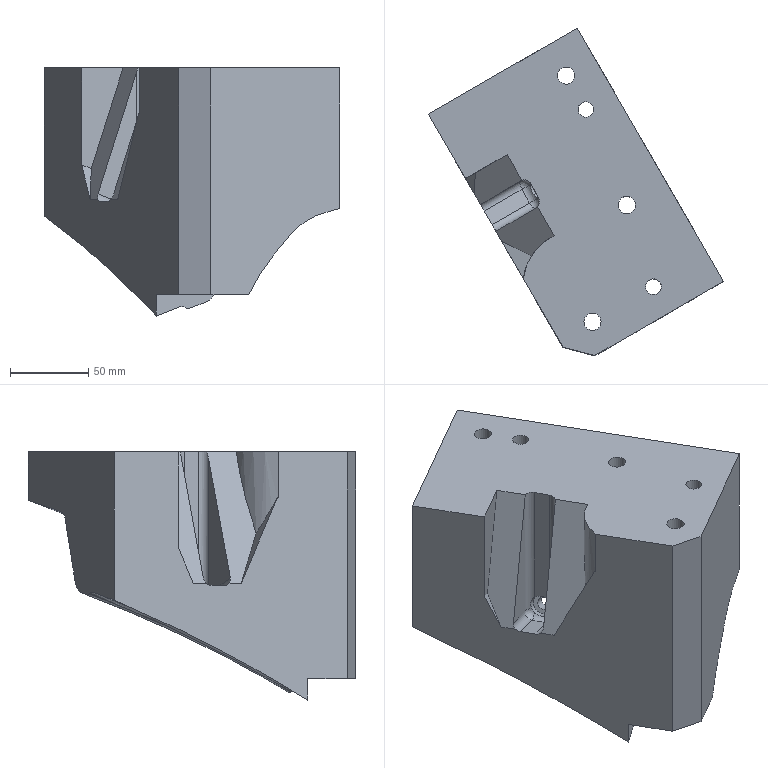Part | NX | features solid 2 | 1 solid | 58 faces | box 188.763 x 209.447 x 158.774 mm | volume 1738141 mm3 | plane 21 | spline 19 | cylinder 16 | sphere 2 | commonest cylinder face diameters 10 x7 11 x3 17 x3 8.1 x1 14 x1 70 x1